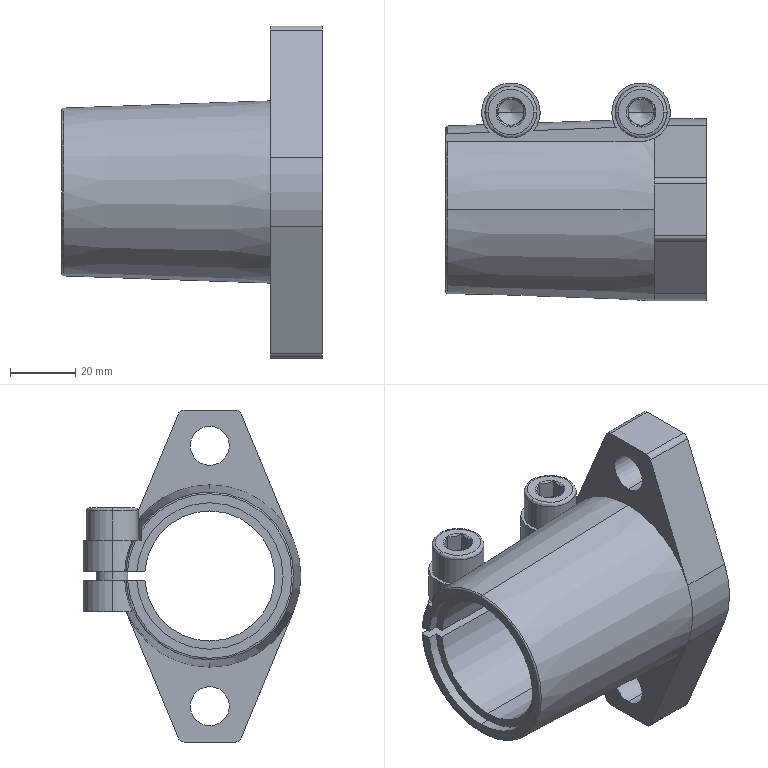Part | STEP file | SHFML40 | 3 solids | 157 faces | box 80 x 67 x 102 mm | volume 113573 mm3 | cone 47 | cylinder 47 | plane 42 | spline 21 | commonest cylinder face diameters 18 x13 8.376 x8 4 x4 10 x4 12 x4 16 x4